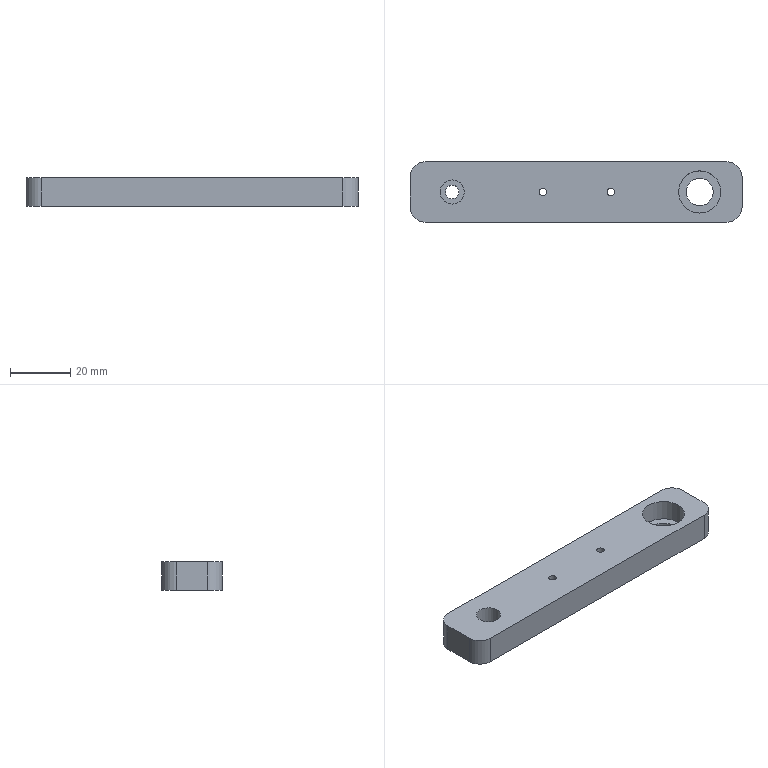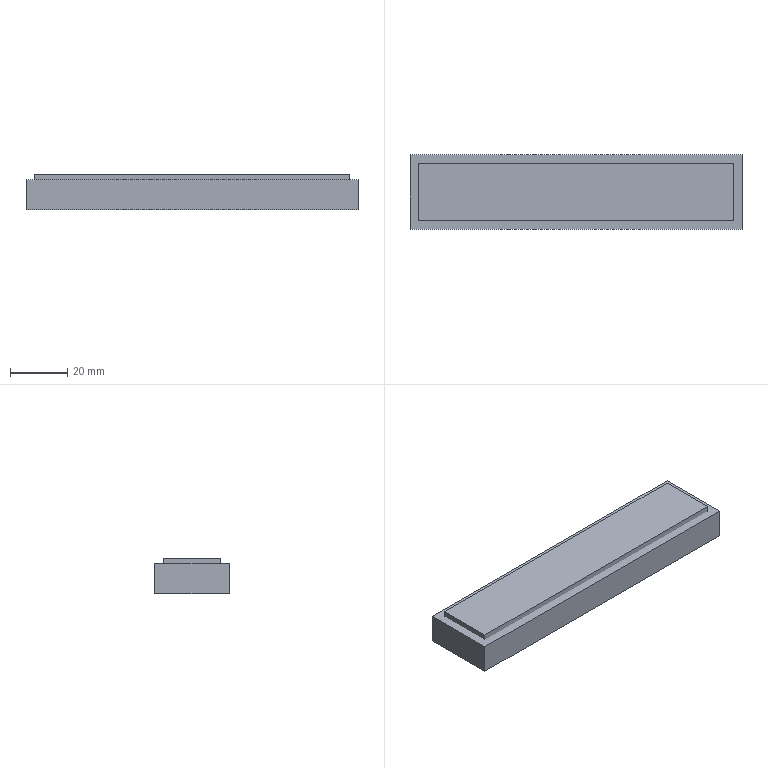CAM job | NX | 3-axis milling, drilling | part box 110 x 20 x 9.5 mm | stock box 116 x 26 x 12.5 mm
Tools:
number,name,description,diameter,corner_radius,flute_length,length,flutes
1,D63,Milling Tool-5 Parameters,63.0,0.0,50.0,75.0,2
9,D6A45,Milling Tool-5 Parameters,6.0,0.0,3.0,3.0,2
14,4.5ZT,Drilling Tool,4.5,0.0,35.0,50.0,2
16,3.1ZT,Drilling Tool,2.0,0.0,35.0,50.0,2
2,D10,Milling Tool-5 Parameters,10.0,0.0,50.0,75.0,2
4,D6,Milling Tool-5 Parameters,6.0,0.0,50.0,75.0,2
Operations:
program,operation,operation_type,tool,method,geometry_group,spindle_rpm,surface_speed,feed_per_tooth,feed_cut,feed_plunge,cut_length_mm,path_length_mm,cut_time_min,machine_time_min
1-115-25-12毛胚-虎钳,FLOOR_WALL,VolumeBased25DMillingOperation,D63,METHOD,A,6500.0,0.0,0.0,1250.0,100.0,191.0,245.0,0.1528,0.1582
1-115-25-12毛胚-虎钳,DRILLING,Operation,D6A45,METHOD,A,4000.0,75.0,0.0312,250.0,0.0,16.0,183.501,0.064,0.0808
1-115-25-12毛胚-虎钳,DRILLING_COPY,Operation,4.5ZT,METHOD,A,2000.0,20.0,0.05,200.0,0.0,30.704,206.463,0.1535,0.1711
1-115-25-12毛胚-虎钳,DRILLING_COPY_COPY,Operation,3.1ZT,METHOD,A,2000.0,20.0,0.05,200.0,0.0,29.202,144.103,0.146,0.1575
1-115-25-12毛胚-虎钳,ADAPTIVE_MILLING,CavityMilling,D10,METHOD,A,7000.0,219.0,0.1429,2000.0,1000.0,1177.419,1250.419,0.5902,0.5975
1-115-25-12毛胚-虎钳,ZLEVEL_PROFILE_COPY_COPY_1_COPY,ZLevelMilling,D10,METHOD,A,6500.0,326.0,0.0769,1000.0,1000.0,291.952,367.952,0.292,0.2996
1-115-25-12毛胚-虎钳,HOLE_MILLING,CylinderMilling,D10,METHOD,A,7000.0,219.0,0.1,1400.0,100.0,113.395,179.895,0.081,0.0876
1-115-25-12毛胚-虎钳,HOLE_MILLING_COPY,CylinderMilling,D6,METHOD,A,7000.0,219.0,0.1,1400.0,100.0,103.971,170.47,0.0743,0.0809
1-115-25-12毛胚-虎钳,HOLE_MILLING_COPY_COPY,CylinderMilling,D6,METHOD,A,7000.0,219.0,0.1,1400.0,100.0,70.765,146.765,0.0505,0.0581
1-115-25-12毛胚-虎钳,ZLEVEL_PROFILE_COPY_1_COPY_COPY_COPY_COPY_COPY_COPY,ZLevelMilling,D6A45,METHOD,A,7000.0,131.0,0.0714,1000.0,1000.0,332.051,890.137,0.3321,0.3879
2-115-25-12毛胚-虎钳,FLOOR_WALL_COPY,VolumeBased25DMillingOperation,D63,METHOD,B,6500.0,0.0,0.0,1250.0,100.0,555.0,1069.001,0.444,0.4954
2-115-25-12毛胚-虎钳,ZLEVEL_PROFILE_COPY_1_COPY_COPY_COPY_COPY_COPY_COPY_COPY,ZLevelMilling,D6A45,METHOD,B,7000.0,131.0,0.0714,1000.0,1000.0,304.255,787.462,0.3043,0.3526